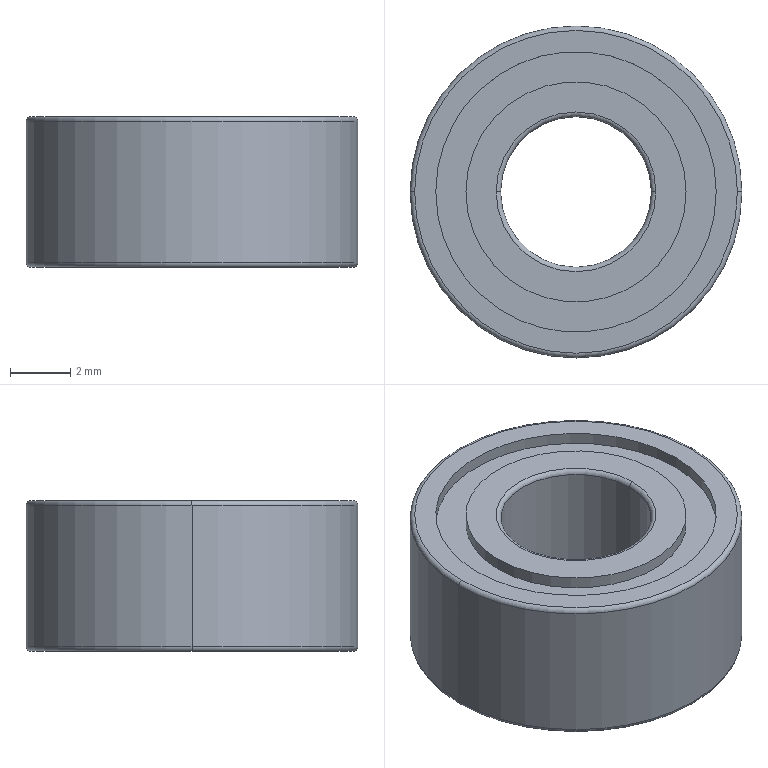Part | 1 solid | 56 faces | box 11 x 11 x 5 mm | volume 259.558 mm3 | sphere 24 | cylinder 16 | torus 8 | plane 8 | commonest cylinder face diameters 7.3 x6 9.3 x6 5 x2 11 x2